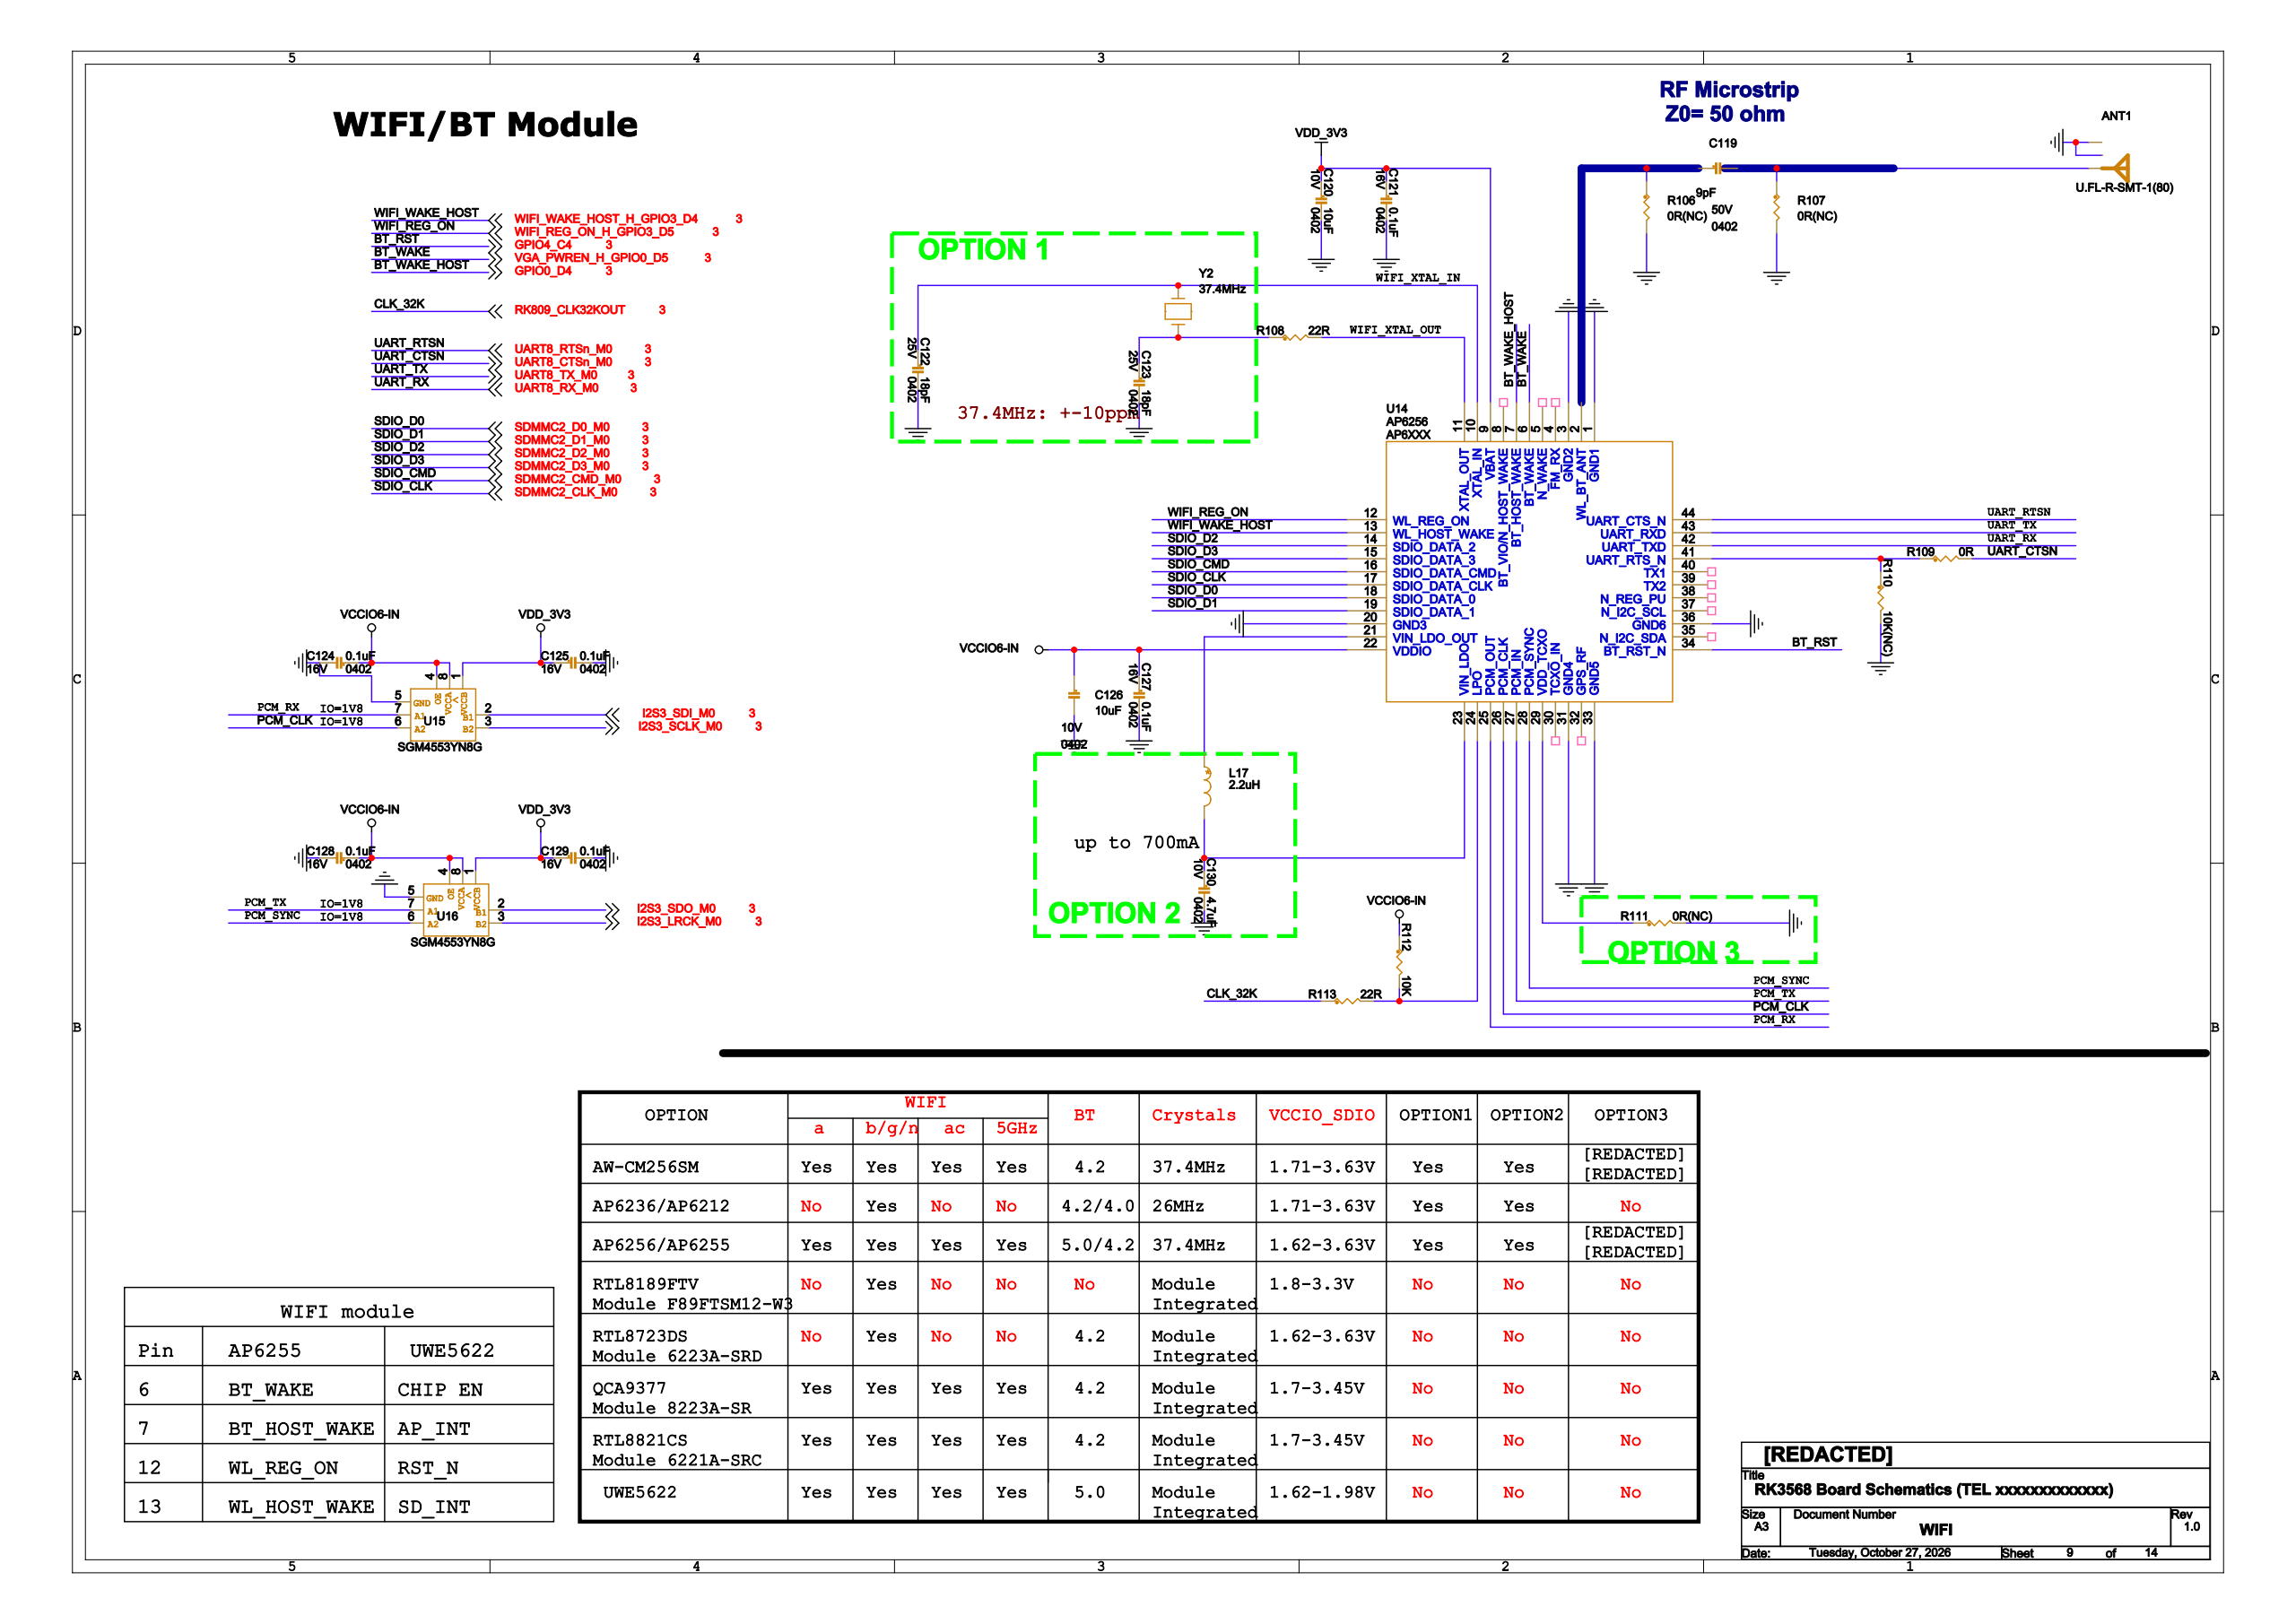Circuit board | Cadence Allegro | 669 parts | 581 nets | one sheet of the schematic
Parts on this sheet (reference | value | footprint):
ANT1 | U.FL-R-SMT-1(80) | IPEX
C119 | 9pF | C0402
C121 | 0.1uF | C0402
C122 | 18pF | C0402
C123 | 18pF | C0402
C124 | 0.1uF | C0402
C125 | 0.1uF | C0402
C126 | 10uF | C0402
C127 | 0.1uF | C0402
C128 | 0.1uF | C0402
C129 | 0.1uF | C0402
C130 | 4.7uF | C0402
L17 | 2.2uH | L2520
R106 | 0R(NC) | R0402
R107 | 0R(NC) | R0402
R108 | 22R | R0402
R109 | 0R | R0402
R110 | 10K(NC) | R0402
R111 | 0R(NC) | R0402
R112 | 10K | R0402
R113 | 22R | R0402
U14 | AP6256 | AP6XXX
U15 | SGM4553YN8G | SOT23_8
U16 | SGM4553YN8G | SOT23_8
Y2 | 37.4MHz | X2520
Nets of these parts (net: part-pin ...):
GND: ANT1-2 ANT1-3 C121-2 C122-2 C123-2 C124-2 C125-2 C126-2 C127-2 C128-2 C129-2 C130-2 R106-2 R107-2 R110-2 R111-2 U15-5 U16-5 Y2-2 Y2-4 U14-1 U14-3 U14-20 U14-31 U14-33 U14-36
VCC3V3_SYS: C121-1 C125-1 C129-1 U15-1 U16-1 U14-9
N83843652: ANT1-1 C119-2 R107-1
VCCIO6-IN: C124-1 C126-1 C127-1 C128-1 R112-1 U15-4 U15-8 U16-4 U16-8 U14-22
N83843645: C119-1 R106-1 U14-2
WIFI_XTAL_IN: C122-1 Y2-3 U14-10
N83843222: C123-1 R108-1 Y2-1
N83843804: C130-1 L17-2 U14-23
N83843775: L17-1 U14-21
N83843641: R111-1 U14-29
WIFI_XTAL_OUT: R108-2 U14-11
RK809_CLK32KOUT: R113-1
N83843827: R112-2 R113-2 U14-24
N83843718: R109-1 R110-1 U14-41
UART8_CTSN_M0: R109-2
GPIO0_D4: U14-7
GPIO4_C4: U14-34
VGA_PWREN_H_GPIO0_D5: U14-6
PCM_CLK: U15-6 U14-26
PCM_TX: U16-7 U14-27
PCM_RX: U15-7 U14-25
PCM_SYNC: U16-6 U14-28
SDMMC2_D0_M0: U14-18
SDMMC2_D1_M0: U14-19
SDMMC2_D2_M0: U14-14
SDMMC2_D3_M0: U14-15
SDMMC2_CLK_M0: U14-17
SDMMC2_CMD_M0: U14-16
UART8_TX_M0: U14-43
UART8_RX_M0: U14-42
WIFI_WAKE_HOST_H_GPIO3_D4: U14-13
WIFI_REG_ON_H_GPIO3_D5: U14-12
I2S3_SDI_M0: U15-2
I2S3_SCLK_M0: U15-3
I2S3_SDO_M0: U16-2
I2S3_LRCK_M0: U16-3